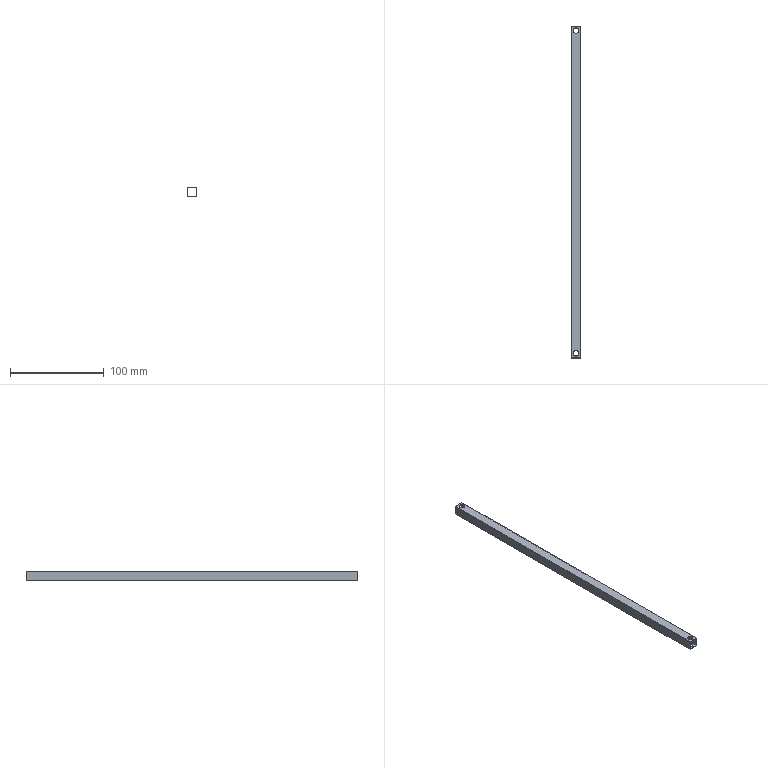Part | SolidWorks | features ICE 2, Extrusion 1 | 1 solid | 18 faces | box 10 x 355 x 10 mm | volume 6688 mm3 | plane 10 | cylinder 8 | commonest cylinder face diameters 6 x8
STEP:
#1=CARTESIAN_POINT('',(-3.,350.,-4.5));
#2=VERTEX_POINT('',#1);
#3=CARTESIAN_POINT('',(3.,350.,-4.5));
#4=VERTEX_POINT('',#3);
#5=CARTESIAN_POINT('',(0.,350.,-4.5));
#6=DIRECTION('',(0.,0.,1.));
#7=DIRECTION('',(1.,0.,0.));
#8=AXIS2_PLACEMENT_3D('',#5,#6,#7);
#9=CIRCLE('',#8,3.);
#10=EDGE_CURVE('',#2,#4,#9,.T.);
#11=ORIENTED_EDGE('',*,*,#10,.T.);
#12=CARTESIAN_POINT('',(3.,350.,-5.));
#13=VERTEX_POINT('',#12);
#14=CARTESIAN_POINT('',(3.,350.,11.));
#15=DIRECTION('',(0.,0.,-1.));
#16=VECTOR('',#15,1000.);
#17=LINE('',#14,#16);
#18=EDGE_CURVE('',#4,#13,#17,.T.);
#19=ORIENTED_EDGE('',*,*,#18,.T.);
#20=CARTESIAN_POINT('',(-3.,350.,-5.));
#21=VERTEX_POINT('',#20);
#22=CARTESIAN_POINT('',(0.,350.,-5.));
#23=DIRECTION('',(0.,0.,-1.));
#24=DIRECTION('',(-1.,0.,0.));
#25=AXIS2_PLACEMENT_3D('',#22,#23,#24);
#26=CIRCLE('',#25,3.);
#27=EDGE_CURVE('',#13,#21,#26,.T.);
#28=ORIENTED_EDGE('',*,*,#27,.T.);
#29=CARTESIAN_POINT('',(-3.,350.,11.));
#30=DIRECTION('',(0.,0.,-1.));
#31=VECTOR('',#30,1000.);
#32=LINE('',#29,#31);
#33=EDGE_CURVE('',#2,#21,#32,.T.);
#34=ORIENTED_EDGE('',*,*,#33,.F.);
#35=EDGE_LOOP('',(#11,#19,#28,#34));
#36=FACE_OUTER_BOUND('',#35,.T.);
#37=CARTESIAN_POINT('',(0.,350.,11.));
#38=DIRECTION('',(0.,0.,-1.));
#39=DIRECTION('',(-1.,0.,0.));
#40=AXIS2_PLACEMENT_3D('',#37,#38,#39);
#41=CYLINDRICAL_SURFACE('',#40,3.);
#42=ADVANCED_FACE('',(#36),#41,.F.);
#43=CARTESIAN_POINT('',(3.,350.,5.));
#44=VERTEX_POINT('',#43);
#45=CARTESIAN_POINT('',(-3.,350.,5.));
#46=VERTEX_POINT('',#45);
#47=CARTESIAN_POINT('',(0.,350.,5.));
#48=DIRECTION('',(0.,0.,-1.));
#49=DIRECTION('',(-1.,0.,0.));
#50=AXIS2_PLACEMENT_3D('',#47,#48,#49);
#51=CIRCLE('',#50,3.);
#52=EDGE_CURVE('',#44,#46,#51,.T.);
#53=ORIENTED_EDGE('',*,*,#52,.F.);
#54=CARTESIAN_POINT('',(3.,350.,4.5));
#55=VERTEX_POINT('',#54);
#56=CARTESIAN_POINT('',(3.,350.,11.));
#57=DIRECTION('',(0.,0.,-1.));
#58=VECTOR('',#57,1000.);
#59=LINE('',#56,#58);
#60=EDGE_CURVE('',#44,#55,#59,.T.);
#61=ORIENTED_EDGE('',*,*,#60,.T.);
#62=CARTESIAN_POINT('',(-3.,350.,4.5));
#63=VERTEX_POINT('',#62);
#64=CARTESIAN_POINT('',(0.,350.,4.5));
#65=DIRECTION('',(0.,0.,-1.));
#66=DIRECTION('',(-1.,0.,0.));
#67=AXIS2_PLACEMENT_3D('',#64,#65,#66);
#68=CIRCLE('',#67,3.);
#69=EDGE_CURVE('',#55,#63,#68,.T.);
#70=ORIENTED_EDGE('',*,*,#69,.T.);
#71=CARTESIAN_POINT('',(-3.,350.,11.));
#72=DIRECTION('',(0.,0.,-1.));
#73=VECTOR('',#72,1000.);
#74=LINE('',#71,#73);
#75=EDGE_CURVE('',#46,#63,#74,.T.);
#76=ORIENTED_EDGE('',*,*,#75,.F.);
#77=EDGE_LOOP('',(#53,#61,#70,#76));
#78=FACE_OUTER_BOUND('',#77,.T.);
#79=CARTESIAN_POINT('',(0.,350.,11.));
#80=DIRECTION('',(0.,0.,-1.));
#81=DIRECTION('',(-1.,0.,0.));
#82=AXIS2_PLACEMENT_3D('',#79,#80,#81);
#83=CYLINDRICAL_SURFACE('',#82,3.);
#84=ADVANCED_FACE('',(#78),#83,.F.);
#85=CARTESIAN_POINT('',(-3.,5.,-4.5));
#86=VERTEX_POINT('',#85);
#87=CARTESIAN_POINT('',(3.,5.,-4.5));
#88=VERTEX_POINT('',#87);
#89=CARTESIAN_POINT('',(0.,5.,-4.5));
#90=DIRECTION('',(0.,0.,1.));
#91=DIRECTION('',(1.,0.,0.));
#92=AXIS2_PLACEMENT_3D('',#89,#90,#91);
#93=CIRCLE('',#92,3.);
#94=EDGE_CURVE('',#86,#88,#93,.T.);
#95=ORIENTED_EDGE('',*,*,#94,.T.);
#96=CARTESIAN_POINT('',(3.,5.,-5.));
#97=VERTEX_POINT('',#96);
#98=CARTESIAN_POINT('',(3.,5.,14.));
#99=DIRECTION('',(0.,0.,-1.));
#100=VECTOR('',#99,1000.);
#101=LINE('',#98,#100);
#102=EDGE_CURVE('',#88,#97,#101,.T.);
#103=ORIENTED_EDGE('',*,*,#102,.T.);
#104=CARTESIAN_POINT('',(-3.,5.,-5.));
#105=VERTEX_POINT('',#104);
#106=CARTESIAN_POINT('',(0.,5.,-5.));
#107=DIRECTION('',(0.,0.,-1.));
#108=DIRECTION('',(-1.,0.,0.));
#109=AXIS2_PLACEMENT_3D('',#106,#107,#108);
#110=CIRCLE('',#109,3.);
#111=EDGE_CURVE('',#97,#105,#110,.T.);
#112=ORIENTED_EDGE('',*,*,#111,.T.);
#113=CARTESIAN_POINT('',(-3.,5.,14.));
#114=DIRECTION('',(0.,0.,-1.));
#115=VECTOR('',#114,1000.);
#116=LINE('',#113,#115);
#117=EDGE_CURVE('',#86,#105,#116,.T.);
#118=ORIENTED_EDGE('',*,*,#117,.F.);
#119=EDGE_LOOP('',(#95,#103,#112,#118));
#120=FACE_OUTER_BOUND('',#119,.T.);
#121=CARTESIAN_POINT('',(0.,5.,14.));
#122=DIRECTION('',(0.,0.,-1.));
#123=DIRECTION('',(-1.,0.,0.));
#124=AXIS2_PLACEMENT_3D('',#121,#122,#123);
#125=CYLINDRICAL_SURFACE('',#124,3.);
#126=ADVANCED_FACE('',(#120),#125,.F.);
#127=CARTESIAN_POINT('',(3.,5.,5.));
#128=VERTEX_POINT('',#127);
#129=CARTESIAN_POINT('',(-3.,5.,5.));
#130=VERTEX_POINT('',#129);
#131=CARTESIAN_POINT('',(0.,5.,5.));
#132=DIRECTION('',(0.,0.,-1.));
#133=DIRECTION('',(-1.,0.,0.));
#134=AXIS2_PLACEMENT_3D('',#131,#132,#133);
#135=CIRCLE('',#134,3.);
#136=EDGE_CURVE('',#128,#130,#135,.T.);
#137=ORIENTED_EDGE('',*,*,#136,.F.);
#138=CARTESIAN_POINT('',(3.,5.,4.5));
#139=VERTEX_POINT('',#138);
#140=CARTESIAN_POINT('',(3.,5.,14.));
#141=DIRECTION('',(0.,0.,-1.));
#142=VECTOR('',#141,1000.);
#143=LINE('',#140,#142);
#144=EDGE_CURVE('',#128,#139,#143,.T.);
#145=ORIENTED_EDGE('',*,*,#144,.T.);
#146=CARTESIAN_POINT('',(-3.,5.,4.5));
#147=VERTEX_POINT('',#146);
#148=CARTESIAN_POINT('',(0.,5.,4.5));
#149=DIRECTION('',(0.,0.,-1.));
#150=DIRECTION('',(-1.,0.,0.));
#151=AXIS2_PLACEMENT_3D('',#148,#149,#150);
#152=CIRCLE('',#151,3.);
#153=EDGE_CURVE('',#139,#147,#152,.T.);
#154=ORIENTED_EDGE('',*,*,#153,.T.);
#155=CARTESIAN_POINT('',(-3.,5.,14.));
#156=DIRECTION('',(0.,0.,-1.));
#157=VECTOR('',#156,1000.);
#158=LINE('',#155,#157);
#159=EDGE_CURVE('',#130,#147,#158,.T.);
#160=ORIENTED_EDGE('',*,*,#159,.F.);
#161=EDGE_LOOP('',(#137,#145,#154,#160));
#162=FACE_OUTER_BOUND('',#161,.T.);
#163=CARTESIAN_POINT('',(0.,5.,14.));
#164=DIRECTION('',(0.,0.,-1.));
#165=DIRECTION('',(-1.,0.,0.));
#166=AXIS2_PLACEMENT_3D('',#163,#164,#165);
#167=CYLINDRICAL_SURFACE('',#166,3.);
#168=ADVANCED_FACE('',(#162),#167,.F.);
#169=CARTESIAN_POINT('',(5.,355.,5.));
#170=VERTEX_POINT('',#169);
#171=CARTESIAN_POINT('',(5.,355.,-5.));
#172=VERTEX_POINT('',#171);
#173=CARTESIAN_POINT('',(5.,355.,-5.));
#174=DIRECTION('',(0.,0.,-1.));
#175=VECTOR('',#174,1000.);
#176=LINE('',#173,#175);
#177=EDGE_CURVE('',#170,#172,#176,.T.);
#178=ORIENTED_EDGE('',*,*,#177,.T.);
#179=CARTESIAN_POINT('',(-5.,355.,-5.));
#180=VERTEX_POINT('',#179);
#181=CARTESIAN_POINT('',(-5.,355.,-5.));
#182=DIRECTION('',(-1.,0.,0.));
#183=VECTOR('',#182,1000.);
#184=LINE('',#181,#183);
#185=EDGE_CURVE('',#172,#180,#184,.T.);
#186=ORIENTED_EDGE('',*,*,#185,.T.);
#187=CARTESIAN_POINT('',(-5.,355.,5.));
#188=VERTEX_POINT('',#187);
#189=CARTESIAN_POINT('',(-5.,355.,-5.));
#190=DIRECTION('',(0.,0.,1.));
#191=VECTOR('',#190,1000.);
#192=LINE('',#189,#191);
#193=EDGE_CURVE('',#180,#188,#192,.T.);
#194=ORIENTED_EDGE('',*,*,#193,.T.);
#195=CARTESIAN_POINT('',(-5.,355.,5.));
#196=DIRECTION('',(1.,0.,0.));
#197=VECTOR('',#196,1000.);
#198=LINE('',#195,#197);
#199=EDGE_CURVE('',#188,#170,#198,.T.);
#200=ORIENTED_EDGE('',*,*,#199,.T.);
#201=EDGE_LOOP('',(#178,#186,#194,#200));
#202=FACE_OUTER_BOUND('',#201,.T.);
#203=CARTESIAN_POINT('',(-4.5,355.,-4.5));
#204=VERTEX_POINT('',#203);
#205=CARTESIAN_POINT('',(-4.5,355.,4.5));
#206=VERTEX_POINT('',#205);
#207=CARTESIAN_POINT('',(-4.5,355.,-4.5));
#208=DIRECTION('',(0.,0.,1.));
#209=VECTOR('',#208,1000.);
#210=LINE('',#207,#209);
#211=EDGE_CURVE('',#204,#206,#210,.T.);
#212=ORIENTED_EDGE('',*,*,#211,.F.);
#213=CARTESIAN_POINT('',(4.5,355.,-4.5));
#214=VERTEX_POINT('',#213);
#215=CARTESIAN_POINT('',(-4.5,355.,-4.5));
#216=DIRECTION('',(-1.,0.,0.));
#217=VECTOR('',#216,1000.);
#218=LINE('',#215,#217);
#219=EDGE_CURVE('',#214,#204,#218,.T.);
#220=ORIENTED_EDGE('',*,*,#219,.F.);
#221=CARTESIAN_POINT('',(4.5,355.,4.5));
#222=VERTEX_POINT('',#221);
#223=CARTESIAN_POINT('',(4.5,355.,-4.5));
#224=DIRECTION('',(0.,0.,-1.));
#225=VECTOR('',#224,1000.);
#226=LINE('',#223,#225);
#227=EDGE_CURVE('',#222,#214,#226,.T.);
#228=ORIENTED_EDGE('',*,*,#227,.F.);
#229=CARTESIAN_POINT('',(-4.5,355.,4.5));
#230=DIRECTION('',(1.,0.,0.));
#231=VECTOR('',#230,1000.);
#232=LINE('',#229,#231);
#233=EDGE_CURVE('',#206,#222,#232,.T.);
#234=ORIENTED_EDGE('',*,*,#233,.F.);
#235=EDGE_LOOP('',(#212,#220,#228,#234));
#236=FACE_BOUND('',#235,.T.);
#237=CARTESIAN_POINT('',(0.,355.,0.));
#238=DIRECTION('',(0.,1.,0.));
#239=DIRECTION('',(0.,0.,1.));
#240=AXIS2_PLACEMENT_3D('',#237,#238,#239);
#241=PLANE('',#240);
#242=ADVANCED_FACE('',(#202,#236),#241,.T.);
#243=CARTESIAN_POINT('',(5.,0.,5.));
#244=VERTEX_POINT('',#243);
#245=CARTESIAN_POINT('',(5.,0.,-5.));
#246=VERTEX_POINT('',#245);
#247=CARTESIAN_POINT('',(5.,0.,-5.));
#248=DIRECTION('',(0.,0.,-1.));
#249=VECTOR('',#248,1000.);
#250=LINE('',#247,#249);
#251=EDGE_CURVE('',#244,#246,#250,.T.);
#252=ORIENTED_EDGE('',*,*,#251,.F.);
#253=CARTESIAN_POINT('',(-5.,0.,5.));
#254=VERTEX_POINT('',#253);
#255=CARTESIAN_POINT('',(-5.,0.,5.));
#256=DIRECTION('',(1.,0.,0.));
#257=VECTOR('',#256,1000.);
#258=LINE('',#255,#257);
#259=EDGE_CURVE('',#254,#244,#258,.T.);
#260=ORIENTED_EDGE('',*,*,#259,.F.);
#261=CARTESIAN_POINT('',(-5.,0.,-5.));
#262=VERTEX_POINT('',#261);
#263=CARTESIAN_POINT('',(-5.,0.,-5.));
#264=DIRECTION('',(0.,0.,1.));
#265=VECTOR('',#264,1000.);
#266=LINE('',#263,#265);
#267=EDGE_CURVE('',#262,#254,#266,.T.);
#268=ORIENTED_EDGE('',*,*,#267,.F.);
#269=CARTESIAN_POINT('',(-5.,0.,-5.));
#270=DIRECTION('',(-1.,0.,0.));
#271=VECTOR('',#270,1000.);
#272=LINE('',#269,#271);
#273=EDGE_CURVE('',#246,#262,#272,.T.);
#274=ORIENTED_EDGE('',*,*,#273,.F.);
#275=EDGE_LOOP('',(#252,#260,#268,#274));
#276=FACE_OUTER_BOUND('',#275,.T.);
#277=CARTESIAN_POINT('',(4.5,0.,-4.5));
#278=VERTEX_POINT('',#277);
#279=CARTESIAN_POINT('',(-4.5,0.,-4.5));
#280=VERTEX_POINT('',#279);
#281=CARTESIAN_POINT('',(-4.5,0.,-4.5));
#282=DIRECTION('',(-1.,0.,0.));
#283=VECTOR('',#282,1000.);
#284=LINE('',#281,#283);
#285=EDGE_CURVE('',#278,#280,#284,.T.);
#286=ORIENTED_EDGE('',*,*,#285,.T.);
#287=CARTESIAN_POINT('',(-4.5,0.,4.5));
#288=VERTEX_POINT('',#287);
#289=CARTESIAN_POINT('',(-4.5,0.,-4.5));
#290=DIRECTION('',(0.,0.,1.));
#291=VECTOR('',#290,1000.);
#292=LINE('',#289,#291);
#293=EDGE_CURVE('',#280,#288,#292,.T.);
#294=ORIENTED_EDGE('',*,*,#293,.T.);
#295=CARTESIAN_POINT('',(4.5,0.,4.5));
#296=VERTEX_POINT('',#295);
#297=CARTESIAN_POINT('',(-4.5,0.,4.5));
#298=DIRECTION('',(1.,0.,0.));
#299=VECTOR('',#298,1000.);
#300=LINE('',#297,#299);
#301=EDGE_CURVE('',#288,#296,#300,.T.);
#302=ORIENTED_EDGE('',*,*,#301,.T.);
#303=CARTESIAN_POINT('',(4.5,0.,-4.5));
#304=DIRECTION('',(0.,0.,-1.));
#305=VECTOR('',#304,1000.);
#306=LINE('',#303,#305);
#307=EDGE_CURVE('',#296,#278,#306,.T.);
#308=ORIENTED_EDGE('',*,*,#307,.T.);
#309=EDGE_LOOP('',(#286,#294,#302,#308));
#310=FACE_BOUND('',#309,.T.);
#311=CARTESIAN_POINT('',(0.,0.,0.));
#312=DIRECTION('',(0.,1.,0.));
#313=DIRECTION('',(0.,0.,1.));
#314=AXIS2_PLACEMENT_3D('',#311,#312,#313);
#315=PLANE('',#314);
#316=ADVANCED_FACE('',(#276,#310),#315,.F.);
#317=ORIENTED_EDGE('',*,*,#251,.T.);
#318=CARTESIAN_POINT('',(5.,355.,-5.));
#319=DIRECTION('',(0.,-1.,0.));
#320=VECTOR('',#319,1000.);
#321=LINE('',#318,#320);
#322=EDGE_CURVE('',#172,#246,#321,.T.);
#323=ORIENTED_EDGE('',*,*,#322,.F.);
#324=ORIENTED_EDGE('',*,*,#177,.F.);
#325=CARTESIAN_POINT('',(5.,355.,5.));
#326=DIRECTION('',(0.,-1.,0.));
#327=VECTOR('',#326,1000.);
#328=LINE('',#325,#327);
#329=EDGE_CURVE('',#170,#244,#328,.T.);
#330=ORIENTED_EDGE('',*,*,#329,.T.);
#331=EDGE_LOOP('',(#317,#323,#324,#330));
#332=FACE_OUTER_BOUND('',#331,.T.);
#333=CARTESIAN_POINT('',(5.,355.,-5.));
#334=DIRECTION('',(-1.,0.,0.));
#335=DIRECTION('',(0.,0.,1.));
#336=AXIS2_PLACEMENT_3D('',#333,#334,#335);
#337=PLANE('',#336);
#338=ADVANCED_FACE('',(#332),#337,.F.);
#339=CARTESIAN_POINT('',(0.,350.,-5.));
#340=DIRECTION('',(0.,0.,-1.));
#341=DIRECTION('',(-1.,0.,0.));
#342=AXIS2_PLACEMENT_3D('',#339,#340,#341);
#343=CIRCLE('',#342,3.);
#344=EDGE_CURVE('',#21,#13,#343,.T.);
#345=ORIENTED_EDGE('',*,*,#344,.F.);
#346=ORIENTED_EDGE('',*,*,#27,.F.);
#347=EDGE_LOOP('',(#345,#346));
#348=FACE_BOUND('',#347,.T.);
#349=CARTESIAN_POINT('',(0.,5.,-5.));
#350=DIRECTION('',(0.,0.,-1.));
#351=DIRECTION('',(-1.,0.,0.));
#352=AXIS2_PLACEMENT_3D('',#349,#350,#351);
#353=CIRCLE('',#352,3.);
#354=EDGE_CURVE('',#105,#97,#353,.T.);
#355=ORIENTED_EDGE('',*,*,#354,.F.);
#356=ORIENTED_EDGE('',*,*,#111,.F.);
#357=EDGE_LOOP('',(#355,#356));
#358=FACE_BOUND('',#357,.T.);
#359=ORIENTED_EDGE('',*,*,#273,.T.);
#360=CARTESIAN_POINT('',(-5.,355.,-5.));
#361=DIRECTION('',(0.,-1.,0.));
#362=VECTOR('',#361,1000.);
#363=LINE('',#360,#362);
#364=EDGE_CURVE('',#180,#262,#363,.T.);
#365=ORIENTED_EDGE('',*,*,#364,.F.);
#366=ORIENTED_EDGE('',*,*,#185,.F.);
#367=ORIENTED_EDGE('',*,*,#322,.T.);
#368=EDGE_LOOP('',(#359,#365,#366,#367));
#369=FACE_OUTER_BOUND('',#368,.T.);
#370=CARTESIAN_POINT('',(-5.,355.,-5.));
#371=DIRECTION('',(0.,0.,1.));
#372=DIRECTION('',(1.,0.,0.));
#373=AXIS2_PLACEMENT_3D('',#370,#371,#372);
#374=PLANE('',#373);
#375=ADVANCED_FACE('',(#348,#358,#369),#374,.F.);
#376=ORIENTED_EDGE('',*,*,#267,.T.);
#377=CARTESIAN_POINT('',(-5.,355.,5.));
#378=DIRECTION('',(0.,-1.,0.));
#379=VECTOR('',#378,1000.);
#380=LINE('',#377,#379);
#381=EDGE_CURVE('',#188,#254,#380,.T.);
#382=ORIENTED_EDGE('',*,*,#381,.F.);
#383=ORIENTED_EDGE('',*,*,#193,.F.);
#384=ORIENTED_EDGE('',*,*,#364,.T.);
#385=EDGE_LOOP('',(#376,#382,#383,#384));
#386=FACE_OUTER_BOUND('',#385,.T.);
#387=CARTESIAN_POINT('',(-5.,355.,-5.));
#388=DIRECTION('',(1.,0.,0.));
#389=DIRECTION('',(0.,0.,-1.));
#390=AXIS2_PLACEMENT_3D('',#387,#388,#389);
#391=PLANE('',#390);
#392=ADVANCED_FACE('',(#386),#391,.F.);
#393=CARTESIAN_POINT('',(0.,350.,5.));
#394=DIRECTION('',(0.,0.,-1.));
#395=DIRECTION('',(-1.,0.,0.));
#396=AXIS2_PLACEMENT_3D('',#393,#394,#395);
#397=CIRCLE('',#396,3.);
#398=EDGE_CURVE('',#46,#44,#397,.T.);
#399=ORIENTED_EDGE('',*,*,#398,.T.);
#400=ORIENTED_EDGE('',*,*,#52,.T.);
#401=EDGE_LOOP('',(#399,#400));
#402=FACE_BOUND('',#401,.T.);
#403=CARTESIAN_POINT('',(0.,5.,5.));
#404=DIRECTION('',(0.,0.,-1.));
#405=DIRECTION('',(-1.,0.,0.));
#406=AXIS2_PLACEMENT_3D('',#403,#404,#405);
#407=CIRCLE('',#406,3.);
#408=EDGE_CURVE('',#130,#128,#407,.T.);
#409=ORIENTED_EDGE('',*,*,#408,.T.);
#410=ORIENTED_EDGE('',*,*,#136,.T.);
#411=EDGE_LOOP('',(#409,#410));
#412=FACE_BOUND('',#411,.T.);
#413=ORIENTED_EDGE('',*,*,#259,.T.);
#414=ORIENTED_EDGE('',*,*,#329,.F.);
#415=ORIENTED_EDGE('',*,*,#199,.F.);
#416=ORIENTED_EDGE('',*,*,#381,.T.);
#417=EDGE_LOOP('',(#413,#414,#415,#416));
#418=FACE_OUTER_BOUND('',#417,.T.);
#419=CARTESIAN_POINT('',(-5.,355.,5.));
#420=DIRECTION('',(0.,0.,-1.));
#421=DIRECTION('',(-1.,0.,0.));
#422=AXIS2_PLACEMENT_3D('',#419,#420,#421);
#423=PLANE('',#422);
#424=ADVANCED_FACE('',(#402,#412,#418),#423,.F.);
#425=ORIENTED_EDGE('',*,*,#10,.F.);
#426=CARTESIAN_POINT('',(0.,350.,-4.5));
#427=DIRECTION('',(0.,0.,1.));
#428=DIRECTION('',(1.,0.,0.));
#429=AXIS2_PLACEMENT_3D('',#426,#427,#428);
#430=CIRCLE('',#429,3.);
#431=EDGE_CURVE('',#4,#2,#430,.T.);
#432=ORIENTED_EDGE('',*,*,#431,.F.);
#433=EDGE_LOOP('',(#425,#432));
#434=FACE_BOUND('',#433,.T.);
#435=ORIENTED_EDGE('',*,*,#94,.F.);
#436=CARTESIAN_POINT('',(0.,5.,-4.5));
#437=DIRECTION('',(0.,0.,1.));
#438=DIRECTION('',(1.,0.,0.));
#439=AXIS2_PLACEMENT_3D('',#436,#437,#438);
#440=CIRCLE('',#439,3.);
#441=EDGE_CURVE('',#88,#86,#440,.T.);
#442=ORIENTED_EDGE('',*,*,#441,.F.);
#443=EDGE_LOOP('',(#435,#442));
#444=FACE_BOUND('',#443,.T.);
#445=ORIENTED_EDGE('',*,*,#285,.F.);
#446=CARTESIAN_POINT('',(4.5,355.,-4.5));
#447=DIRECTION('',(0.,-1.,0.));
#448=VECTOR('',#447,1000.);
#449=LINE('',#446,#448);
#450=EDGE_CURVE('',#214,#278,#449,.T.);
#451=ORIENTED_EDGE('',*,*,#450,.F.);
#452=ORIENTED_EDGE('',*,*,#219,.T.);
#453=CARTESIAN_POINT('',(-4.5,355.,-4.5));
#454=DIRECTION('',(0.,-1.,0.));
#455=VECTOR('',#454,1000.);
#456=LINE('',#453,#455);
#457=EDGE_CURVE('',#204,#280,#456,.T.);
#458=ORIENTED_EDGE('',*,*,#457,.T.);
#459=EDGE_LOOP('',(#445,#451,#452,#458));
#460=FACE_OUTER_BOUND('',#459,.T.);
#461=CARTESIAN_POINT('',(-4.5,355.,-4.5));
#462=DIRECTION('',(0.,0.,1.));
#463=DIRECTION('',(1.,0.,0.));
#464=AXIS2_PLACEMENT_3D('',#461,#462,#463);
#465=PLANE('',#464);
#466=ADVANCED_FACE('',(#434,#444,#460),#465,.T.);
#467=ORIENTED_EDGE('',*,*,#293,.F.);
#468=ORIENTED_EDGE('',*,*,#457,.F.);
#469=ORIENTED_EDGE('',*,*,#211,.T.);
#470=CARTESIAN_POINT('',(-4.5,355.,4.5));
#471=DIRECTION('',(0.,-1.,0.));
#472=VECTOR('',#471,1000.);
#473=LINE('',#470,#472);
#474=EDGE_CURVE('',#206,#288,#473,.T.);
#475=ORIENTED_EDGE('',*,*,#474,.T.);
#476=EDGE_LOOP('',(#467,#468,#469,#475));
#477=FACE_OUTER_BOUND('',#476,.T.);
#478=CARTESIAN_POINT('',(-4.5,355.,-4.5));
#479=DIRECTION('',(1.,0.,0.));
#480=DIRECTION('',(0.,0.,-1.));
#481=AXIS2_PLACEMENT_3D('',#478,#479,#480);
#482=PLANE('',#481);
#483=ADVANCED_FACE('',(#477),#482,.T.);
#484=CARTESIAN_POINT('',(0.,350.,4.5));
#485=DIRECTION('',(0.,0.,-1.));
#486=DIRECTION('',(-1.,0.,0.));
#487=AXIS2_PLACEMENT_3D('',#484,#485,#486);
#488=CIRCLE('',#487,3.);
#489=EDGE_CURVE('',#63,#55,#488,.T.);
#490=ORIENTED_EDGE('',*,*,#489,.F.);
#491=ORIENTED_EDGE('',*,*,#69,.F.);
#492=EDGE_LOOP('',(#490,#491));
#493=FACE_BOUND('',#492,.T.);
#494=CARTESIAN_POINT('',(0.,5.,4.5));
#495=DIRECTION('',(0.,0.,-1.));
#496=DIRECTION('',(-1.,0.,0.));
#497=AXIS2_PLACEMENT_3D('',#494,#495,#496);
#498=CIRCLE('',#497,3.);
#499=EDGE_CURVE('',#147,#139,#498,.T.);
#500=ORIENTED_EDGE('',*,*,#499,.F.);
#501=ORIENTED_EDGE('',*,*,#153,.F.);
#502=EDGE_LOOP('',(#500,#501));
#503=FACE_BOUND('',#502,.T.);
#504=ORIENTED_EDGE('',*,*,#301,.F.);
#505=ORIENTED_EDGE('',*,*,#474,.F.);
#506=ORIENTED_EDGE('',*,*,#233,.T.);
#507=CARTESIAN_POINT('',(4.5,355.,4.5));
#508=DIRECTION('',(0.,-1.,0.));
#509=VECTOR('',#508,1000.);
#510=LINE('',#507,#509);
#511=EDGE_CURVE('',#222,#296,#510,.T.);
#512=ORIENTED_EDGE('',*,*,#511,.T.);
#513=EDGE_LOOP('',(#504,#505,#506,#512));
#514=FACE_OUTER_BOUND('',#513,.T.);
#515=CARTESIAN_POINT('',(-4.5,355.,4.5));
#516=DIRECTION('',(0.,0.,-1.));
#517=DIRECTION('',(-1.,0.,0.));
#518=AXIS2_PLACEMENT_3D('',#515,#516,#517);
#519=PLANE('',#518);
#520=ADVANCED_FACE('',(#493,#503,#514),#519,.T.);
#521=ORIENTED_EDGE('',*,*,#307,.F.);
#522=ORIENTED_EDGE('',*,*,#511,.F.);
#523=ORIENTED_EDGE('',*,*,#227,.T.);
#524=ORIENTED_EDGE('',*,*,#450,.T.);
#525=EDGE_LOOP('',(#521,#522,#523,#524));
#526=FACE_OUTER_BOUND('',#525,.T.);
#527=CARTESIAN_POINT('',(4.5,355.,-4.5));
#528=DIRECTION('',(-1.,0.,0.));
#529=DIRECTION('',(0.,0.,1.));
#530=AXIS2_PLACEMENT_3D('',#527,#528,#529);
#531=PLANE('',#530);
#532=ADVANCED_FACE('',(#526),#531,.T.);
#533=ORIENTED_EDGE('',*,*,#144,.F.);
#534=ORIENTED_EDGE('',*,*,#408,.F.);
#535=ORIENTED_EDGE('',*,*,#159,.T.);
#536=ORIENTED_EDGE('',*,*,#499,.T.);
#537=EDGE_LOOP('',(#533,#534,#535,#536));
#538=FACE_OUTER_BOUND('',#537,.T.);
#539=CARTESIAN_POINT('',(0.,5.,14.));
#540=DIRECTION('',(0.,0.,-1.));
#541=DIRECTION('',(-1.,0.,0.));
#542=AXIS2_PLACEMENT_3D('',#539,#540,#541);
#543=CYLINDRICAL_SURFACE('',#542,3.);
#544=ADVANCED_FACE('',(#538),#543,.F.);
#545=ORIENTED_EDGE('',*,*,#102,.F.);
#546=ORIENTED_EDGE('',*,*,#441,.T.);
#547=ORIENTED_EDGE('',*,*,#117,.T.);
#548=ORIENTED_EDGE('',*,*,#354,.T.);
#549=EDGE_LOOP('',(#545,#546,#547,#548));
#550=FACE_OUTER_BOUND('',#549,.T.);
#551=CARTESIAN_POINT('',(0.,5.,14.));
#552=DIRECTION('',(0.,0.,-1.));
#553=DIRECTION('',(-1.,0.,0.));
#554=AXIS2_PLACEMENT_3D('',#551,#552,#553);
#555=CYLINDRICAL_SURFACE('',#554,3.);
#556=ADVANCED_FACE('',(#550),#555,.F.);
#557=ORIENTED_EDGE('',*,*,#60,.F.);
#558=ORIENTED_EDGE('',*,*,#398,.F.);
#559=ORIENTED_EDGE('',*,*,#75,.T.);
#560=ORIENTED_EDGE('',*,*,#489,.T.);
#561=EDGE_LOOP('',(#557,#558,#559,#560));
#562=FACE_OUTER_BOUND('',#561,.T.);
#563=CARTESIAN_POINT('',(0.,350.,11.));
#564=DIRECTION('',(0.,0.,-1.));
#565=DIRECTION('',(-1.,0.,0.));
#566=AXIS2_PLACEMENT_3D('',#563,#564,#565);
#567=CYLINDRICAL_SURFACE('',#566,3.);
#568=ADVANCED_FACE('',(#562),#567,.F.);
#569=ORIENTED_EDGE('',*,*,#18,.F.);
#570=ORIENTED_EDGE('',*,*,#431,.T.);
#571=ORIENTED_EDGE('',*,*,#33,.T.);
#572=ORIENTED_EDGE('',*,*,#344,.T.);
#573=EDGE_LOOP('',(#569,#570,#571,#572));
#574=FACE_OUTER_BOUND('',#573,.T.);
#575=CARTESIAN_POINT('',(0.,350.,11.));
#576=DIRECTION('',(0.,0.,-1.));
#577=DIRECTION('',(-1.,0.,0.));
#578=AXIS2_PLACEMENT_3D('',#575,#576,#577);
#579=CYLINDRICAL_SURFACE('',#578,3.);
#580=ADVANCED_FACE('',(#574),#579,.F.);
#581=CLOSED_SHELL('',(#42,#84,#126,#168,#242,#316,#338,#375,#392,#424,#466,#483,#520,#532,#544,#556,#568,#580));
#582=MANIFOLD_SOLID_BREP('',#581);
#583=CARTESIAN_POINT('',(0.,0.,0.));
#584=DIRECTION('',(0.,0.,1.));
#585=DIRECTION('',(1.,0.,0.));
#586=AXIS2_PLACEMENT_3D('',#583,#584,#585);
#587=(LENGTH_UNIT()NAMED_UNIT(*)SI_UNIT(.MILLI.,.METRE.));
#588=UNCERTAINTY_MEASURE_WITH_UNIT(LENGTH_MEASURE(0.00001),#587,'','');
#589=(NAMED_UNIT(*)PLANE_ANGLE_UNIT()SI_UNIT($,.RADIAN.));
#590=(NAMED_UNIT(*)SI_UNIT($,.STERADIAN.)SOLID_ANGLE_UNIT());
#591=(GEOMETRIC_REPRESENTATION_CONTEXT(3)GLOBAL_UNCERTAINTY_ASSIGNED_CONTEXT((#588))GLOBAL_UNIT_ASSIGNED_CONTEXT((#587,#589,#590))REPRESENTATION_CONTEXT('',''));
#592=ADVANCED_BREP_SHAPE_REPRESENTATION('',(#582,#586),#591);